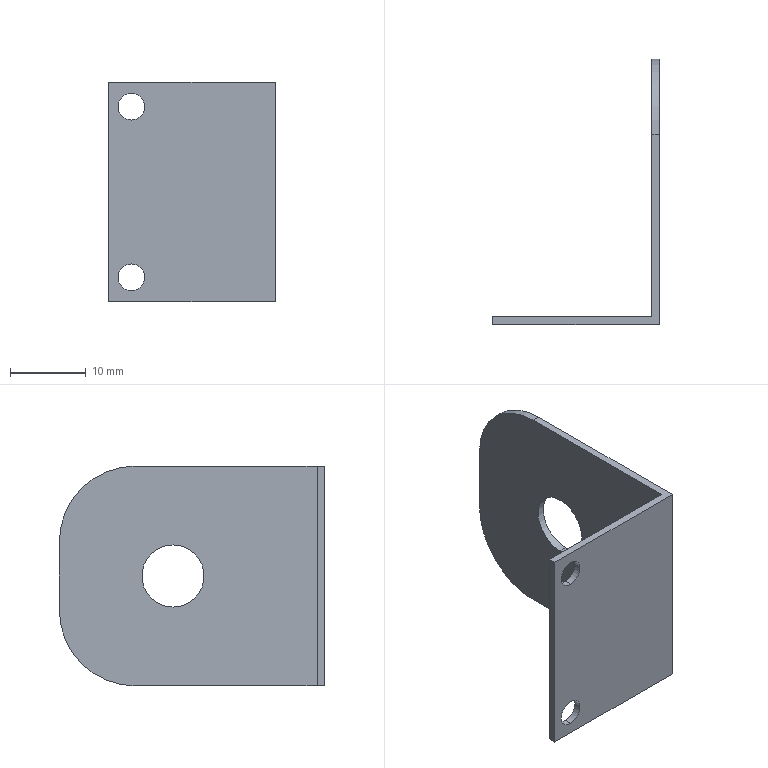Part | 1 solid | 16 faces | box 22 x 35 x 29 mm | volume 1509 mm3 | cylinder 8 | plane 8 | commonest cylinder face diameters 3.5 x4 8.2 x2 20 x2
STEP:
#1=CARTESIAN_POINT('',(10.,20.,4.1));
#2=VERTEX_POINT('',#1);
#3=CARTESIAN_POINT('',(10.,20.,-4.1));
#4=VERTEX_POINT('',#3);
#5=CARTESIAN_POINT('',(10.,20.,0.));
#6=DIRECTION('',(1.,0.,0.));
#7=DIRECTION('',(0.,0.,-1.));
#8=AXIS2_PLACEMENT_3D('',#5,#6,#7);
#9=CIRCLE('',#8,4.1);
#10=EDGE_CURVE('',#2,#4,#9,.T.);
#11=ORIENTED_EDGE('',*,*,#10,.F.);
#12=CARTESIAN_POINT('',(11.,20.,4.1));
#13=VERTEX_POINT('',#12);
#14=CARTESIAN_POINT('',(10.,20.,4.1));
#15=DIRECTION('',(1.,0.,0.));
#16=VECTOR('',#15,1000.);
#17=LINE('',#14,#16);
#18=EDGE_CURVE('',#2,#13,#17,.T.);
#19=ORIENTED_EDGE('',*,*,#18,.T.);
#20=CARTESIAN_POINT('',(11.,20.,-4.1));
#21=VERTEX_POINT('',#20);
#22=CARTESIAN_POINT('',(11.,20.,0.));
#23=DIRECTION('',(1.,0.,0.));
#24=DIRECTION('',(0.,0.,-1.));
#25=AXIS2_PLACEMENT_3D('',#22,#23,#24);
#26=CIRCLE('',#25,4.1);
#27=EDGE_CURVE('',#13,#21,#26,.T.);
#28=ORIENTED_EDGE('',*,*,#27,.T.);
#29=CARTESIAN_POINT('',(10.,20.,-4.1));
#30=DIRECTION('',(1.,0.,0.));
#31=VECTOR('',#30,1000.);
#32=LINE('',#29,#31);
#33=EDGE_CURVE('',#4,#21,#32,.T.);
#34=ORIENTED_EDGE('',*,*,#33,.F.);
#35=EDGE_LOOP('',(#11,#19,#28,#34));
#36=FACE_OUTER_BOUND('',#35,.T.);
#37=CARTESIAN_POINT('',(10.,20.,0.));
#38=DIRECTION('',(1.,0.,0.));
#39=DIRECTION('',(0.,0.,-1.));
#40=AXIS2_PLACEMENT_3D('',#37,#38,#39);
#41=CYLINDRICAL_SURFACE('',#40,4.1);
#42=ADVANCED_FACE('',(#36),#41,.F.);
#43=CARTESIAN_POINT('',(-8.,1.,9.5));
#44=VERTEX_POINT('',#43);
#45=CARTESIAN_POINT('',(-8.,1.,13.));
#46=VERTEX_POINT('',#45);
#47=CARTESIAN_POINT('',(-8.,1.,11.25));
#48=DIRECTION('',(0.,1.,0.));
#49=DIRECTION('',(0.,0.,1.));
#50=AXIS2_PLACEMENT_3D('',#47,#48,#49);
#51=CIRCLE('',#50,1.75);
#52=EDGE_CURVE('',#44,#46,#51,.T.);
#53=ORIENTED_EDGE('',*,*,#52,.T.);
#54=CARTESIAN_POINT('',(-8.,0.,13.));
#55=VERTEX_POINT('',#54);
#56=CARTESIAN_POINT('',(-8.,1.,13.));
#57=DIRECTION('',(0.,-1.,0.));
#58=VECTOR('',#57,1000.);
#59=LINE('',#56,#58);
#60=EDGE_CURVE('',#46,#55,#59,.T.);
#61=ORIENTED_EDGE('',*,*,#60,.T.);
#62=CARTESIAN_POINT('',(-8.,0.,9.5));
#63=VERTEX_POINT('',#62);
#64=CARTESIAN_POINT('',(-8.,0.,11.25));
#65=DIRECTION('',(0.,1.,0.));
#66=DIRECTION('',(0.,0.,1.));
#67=AXIS2_PLACEMENT_3D('',#64,#65,#66);
#68=CIRCLE('',#67,1.75);
#69=EDGE_CURVE('',#63,#55,#68,.T.);
#70=ORIENTED_EDGE('',*,*,#69,.F.);
#71=CARTESIAN_POINT('',(-8.,1.,9.5));
#72=DIRECTION('',(0.,-1.,0.));
#73=VECTOR('',#72,1000.);
#74=LINE('',#71,#73);
#75=EDGE_CURVE('',#44,#63,#74,.T.);
#76=ORIENTED_EDGE('',*,*,#75,.F.);
#77=EDGE_LOOP('',(#53,#61,#70,#76));
#78=FACE_OUTER_BOUND('',#77,.T.);
#79=CARTESIAN_POINT('',(-8.,1.,11.25));
#80=DIRECTION('',(0.,-1.,0.));
#81=DIRECTION('',(0.,0.,-1.));
#82=AXIS2_PLACEMENT_3D('',#79,#80,#81);
#83=CYLINDRICAL_SURFACE('',#82,1.75);
#84=ADVANCED_FACE('',(#78),#83,.F.);
#85=CARTESIAN_POINT('',(-8.,1.,-13.));
#86=VERTEX_POINT('',#85);
#87=CARTESIAN_POINT('',(-8.,1.,-9.5));
#88=VERTEX_POINT('',#87);
#89=CARTESIAN_POINT('',(-8.,1.,-11.25));
#90=DIRECTION('',(0.,1.,0.));
#91=DIRECTION('',(0.,0.,1.));
#92=AXIS2_PLACEMENT_3D('',#89,#90,#91);
#93=CIRCLE('',#92,1.75);
#94=EDGE_CURVE('',#86,#88,#93,.T.);
#95=ORIENTED_EDGE('',*,*,#94,.T.);
#96=CARTESIAN_POINT('',(-8.,0.,-9.5));
#97=VERTEX_POINT('',#96);
#98=CARTESIAN_POINT('',(-8.,1.,-9.5));
#99=DIRECTION('',(0.,-1.,0.));
#100=VECTOR('',#99,1000.);
#101=LINE('',#98,#100);
#102=EDGE_CURVE('',#88,#97,#101,.T.);
#103=ORIENTED_EDGE('',*,*,#102,.T.);
#104=CARTESIAN_POINT('',(-8.,0.,-13.));
#105=VERTEX_POINT('',#104);
#106=CARTESIAN_POINT('',(-8.,0.,-11.25));
#107=DIRECTION('',(0.,1.,0.));
#108=DIRECTION('',(0.,0.,1.));
#109=AXIS2_PLACEMENT_3D('',#106,#107,#108);
#110=CIRCLE('',#109,1.75);
#111=EDGE_CURVE('',#105,#97,#110,.T.);
#112=ORIENTED_EDGE('',*,*,#111,.F.);
#113=CARTESIAN_POINT('',(-8.,1.,-13.));
#114=DIRECTION('',(0.,-1.,0.));
#115=VECTOR('',#114,1000.);
#116=LINE('',#113,#115);
#117=EDGE_CURVE('',#86,#105,#116,.T.);
#118=ORIENTED_EDGE('',*,*,#117,.F.);
#119=EDGE_LOOP('',(#95,#103,#112,#118));
#120=FACE_OUTER_BOUND('',#119,.T.);
#121=CARTESIAN_POINT('',(-8.,1.,-11.25));
#122=DIRECTION('',(0.,-1.,0.));
#123=DIRECTION('',(0.,0.,-1.));
#124=AXIS2_PLACEMENT_3D('',#121,#122,#123);
#125=CYLINDRICAL_SURFACE('',#124,1.75);
#126=ADVANCED_FACE('',(#120),#125,.F.);
#127=CARTESIAN_POINT('',(10.,1.,-14.5));
#128=VERTEX_POINT('',#127);
#129=CARTESIAN_POINT('',(10.,1.,14.5));
#130=VERTEX_POINT('',#129);
#131=CARTESIAN_POINT('',(10.,1.,0.));
#132=DIRECTION('',(0.,0.,1.));
#133=VECTOR('',#132,1000.);
#134=LINE('',#131,#133);
#135=EDGE_CURVE('',#128,#130,#134,.T.);
#136=ORIENTED_EDGE('',*,*,#135,.F.);
#137=CARTESIAN_POINT('',(-11.,1.,-14.5));
#138=VERTEX_POINT('',#137);
#139=CARTESIAN_POINT('',(-11.,1.,-14.5));
#140=DIRECTION('',(-1.,0.,0.));
#141=VECTOR('',#140,1000.);
#142=LINE('',#139,#141);
#143=EDGE_CURVE('',#128,#138,#142,.T.);
#144=ORIENTED_EDGE('',*,*,#143,.T.);
#145=CARTESIAN_POINT('',(-11.,1.,14.5));
#146=VERTEX_POINT('',#145);
#147=CARTESIAN_POINT('',(-11.,1.,-14.5));
#148=DIRECTION('',(0.,0.,1.));
#149=VECTOR('',#148,1000.);
#150=LINE('',#147,#149);
#151=EDGE_CURVE('',#138,#146,#150,.T.);
#152=ORIENTED_EDGE('',*,*,#151,.T.);
#153=CARTESIAN_POINT('',(-11.,1.,14.5));
#154=DIRECTION('',(1.,0.,0.));
#155=VECTOR('',#154,1000.);
#156=LINE('',#153,#155);
#157=EDGE_CURVE('',#146,#130,#156,.T.);
#158=ORIENTED_EDGE('',*,*,#157,.T.);
#159=EDGE_LOOP('',(#136,#144,#152,#158));
#160=FACE_OUTER_BOUND('',#159,.T.);
#161=ORIENTED_EDGE('',*,*,#94,.F.);
#162=CARTESIAN_POINT('',(-8.,1.,-11.25));
#163=DIRECTION('',(0.,1.,0.));
#164=DIRECTION('',(0.,0.,1.));
#165=AXIS2_PLACEMENT_3D('',#162,#163,#164);
#166=CIRCLE('',#165,1.75);
#167=EDGE_CURVE('',#88,#86,#166,.T.);
#168=ORIENTED_EDGE('',*,*,#167,.F.);
#169=EDGE_LOOP('',(#161,#168));
#170=FACE_BOUND('',#169,.T.);
#171=ORIENTED_EDGE('',*,*,#52,.F.);
#172=CARTESIAN_POINT('',(-8.,1.,11.25));
#173=DIRECTION('',(0.,1.,0.));
#174=DIRECTION('',(0.,0.,1.));
#175=AXIS2_PLACEMENT_3D('',#172,#173,#174);
#176=CIRCLE('',#175,1.75);
#177=EDGE_CURVE('',#46,#44,#176,.T.);
#178=ORIENTED_EDGE('',*,*,#177,.F.);
#179=EDGE_LOOP('',(#171,#178));
#180=FACE_BOUND('',#179,.T.);
#181=CARTESIAN_POINT('',(0.,1.,0.));
#182=DIRECTION('',(0.,1.,0.));
#183=DIRECTION('',(0.,0.,1.));
#184=AXIS2_PLACEMENT_3D('',#181,#182,#183);
#185=PLANE('',#184);
#186=ADVANCED_FACE('',(#160,#170,#180),#185,.T.);
#187=CARTESIAN_POINT('',(-11.,0.,-14.5));
#188=VERTEX_POINT('',#187);
#189=CARTESIAN_POINT('',(-11.,0.,14.5));
#190=VERTEX_POINT('',#189);
#191=CARTESIAN_POINT('',(-11.,0.,-14.5));
#192=DIRECTION('',(0.,0.,1.));
#193=VECTOR('',#192,1000.);
#194=LINE('',#191,#193);
#195=EDGE_CURVE('',#188,#190,#194,.T.);
#196=ORIENTED_EDGE('',*,*,#195,.F.);
#197=CARTESIAN_POINT('',(11.,0.,-14.5));
#198=VERTEX_POINT('',#197);
#199=CARTESIAN_POINT('',(-11.,0.,-14.5));
#200=DIRECTION('',(-1.,0.,0.));
#201=VECTOR('',#200,1000.);
#202=LINE('',#199,#201);
#203=EDGE_CURVE('',#198,#188,#202,.T.);
#204=ORIENTED_EDGE('',*,*,#203,.F.);
#205=CARTESIAN_POINT('',(11.,0.,14.5));
#206=VERTEX_POINT('',#205);
#207=CARTESIAN_POINT('',(11.,0.,-14.5));
#208=DIRECTION('',(0.,0.,-1.));
#209=VECTOR('',#208,1000.);
#210=LINE('',#207,#209);
#211=EDGE_CURVE('',#206,#198,#210,.T.);
#212=ORIENTED_EDGE('',*,*,#211,.F.);
#213=CARTESIAN_POINT('',(-11.,0.,14.5));
#214=DIRECTION('',(1.,0.,0.));
#215=VECTOR('',#214,1000.);
#216=LINE('',#213,#215);
#217=EDGE_CURVE('',#190,#206,#216,.T.);
#218=ORIENTED_EDGE('',*,*,#217,.F.);
#219=EDGE_LOOP('',(#196,#204,#212,#218));
#220=FACE_OUTER_BOUND('',#219,.T.);
#221=ORIENTED_EDGE('',*,*,#111,.T.);
#222=CARTESIAN_POINT('',(-8.,0.,-11.25));
#223=DIRECTION('',(0.,1.,0.));
#224=DIRECTION('',(0.,0.,1.));
#225=AXIS2_PLACEMENT_3D('',#222,#223,#224);
#226=CIRCLE('',#225,1.75);
#227=EDGE_CURVE('',#97,#105,#226,.T.);
#228=ORIENTED_EDGE('',*,*,#227,.T.);
#229=EDGE_LOOP('',(#221,#228));
#230=FACE_BOUND('',#229,.T.);
#231=ORIENTED_EDGE('',*,*,#69,.T.);
#232=CARTESIAN_POINT('',(-8.,0.,11.25));
#233=DIRECTION('',(0.,1.,0.));
#234=DIRECTION('',(0.,0.,1.));
#235=AXIS2_PLACEMENT_3D('',#232,#233,#234);
#236=CIRCLE('',#235,1.75);
#237=EDGE_CURVE('',#55,#63,#236,.T.);
#238=ORIENTED_EDGE('',*,*,#237,.T.);
#239=EDGE_LOOP('',(#231,#238));
#240=FACE_BOUND('',#239,.T.);
#241=CARTESIAN_POINT('',(0.,0.,0.));
#242=DIRECTION('',(0.,1.,0.));
#243=DIRECTION('',(0.,0.,1.));
#244=AXIS2_PLACEMENT_3D('',#241,#242,#243);
#245=PLANE('',#244);
#246=ADVANCED_FACE('',(#220,#230,#240),#245,.F.);
#247=CARTESIAN_POINT('',(11.,25.,-14.5));
#248=VERTEX_POINT('',#247);
#249=CARTESIAN_POINT('',(11.,1.,-14.5));
#250=DIRECTION('',(0.,-1.,0.));
#251=VECTOR('',#250,1000.);
#252=LINE('',#249,#251);
#253=EDGE_CURVE('',#248,#198,#252,.T.);
#254=ORIENTED_EDGE('',*,*,#253,.F.);
#255=CARTESIAN_POINT('',(11.,35.,-4.5));
#256=VERTEX_POINT('',#255);
#257=CARTESIAN_POINT('',(11.,25.,-4.5));
#258=DIRECTION('',(1.,0.,0.));
#259=DIRECTION('',(0.,0.,1.));
#260=AXIS2_PLACEMENT_3D('',#257,#258,#259);
#261=CIRCLE('',#260,10.);
#262=EDGE_CURVE('',#248,#256,#261,.T.);
#263=ORIENTED_EDGE('',*,*,#262,.T.);
#264=CARTESIAN_POINT('',(11.,35.,4.5));
#265=VERTEX_POINT('',#264);
#266=CARTESIAN_POINT('',(11.,35.,14.5));
#267=DIRECTION('',(0.,0.,1.));
#268=VECTOR('',#267,1000.);
#269=LINE('',#266,#268);
#270=EDGE_CURVE('',#256,#265,#269,.T.);
#271=ORIENTED_EDGE('',*,*,#270,.T.);
#272=CARTESIAN_POINT('',(11.,25.,14.5));
#273=VERTEX_POINT('',#272);
#274=CARTESIAN_POINT('',(11.,25.,4.5));
#275=DIRECTION('',(1.,0.,0.));
#276=DIRECTION('',(0.,0.,1.));
#277=AXIS2_PLACEMENT_3D('',#274,#275,#276);
#278=CIRCLE('',#277,10.);
#279=EDGE_CURVE('',#265,#273,#278,.T.);
#280=ORIENTED_EDGE('',*,*,#279,.T.);
#281=CARTESIAN_POINT('',(11.,1.,14.5));
#282=DIRECTION('',(0.,-1.,0.));
#283=VECTOR('',#282,1000.);
#284=LINE('',#281,#283);
#285=EDGE_CURVE('',#273,#206,#284,.T.);
#286=ORIENTED_EDGE('',*,*,#285,.T.);
#287=ORIENTED_EDGE('',*,*,#211,.T.);
#288=EDGE_LOOP('',(#254,#263,#271,#280,#286,#287));
#289=FACE_OUTER_BOUND('',#288,.T.);
#290=CARTESIAN_POINT('',(11.,20.,0.));
#291=DIRECTION('',(1.,0.,0.));
#292=DIRECTION('',(0.,0.,-1.));
#293=AXIS2_PLACEMENT_3D('',#290,#291,#292);
#294=CIRCLE('',#293,4.1);
#295=EDGE_CURVE('',#21,#13,#294,.T.);
#296=ORIENTED_EDGE('',*,*,#295,.F.);
#297=ORIENTED_EDGE('',*,*,#27,.F.);
#298=EDGE_LOOP('',(#296,#297));
#299=FACE_BOUND('',#298,.T.);
#300=CARTESIAN_POINT('',(11.,1.,-14.5));
#301=DIRECTION('',(-1.,0.,0.));
#302=DIRECTION('',(0.,0.,1.));
#303=AXIS2_PLACEMENT_3D('',#300,#301,#302);
#304=PLANE('',#303);
#305=ADVANCED_FACE('',(#289,#299),#304,.F.);
#306=CARTESIAN_POINT('',(10.,25.,-14.5));
#307=VERTEX_POINT('',#306);
#308=CARTESIAN_POINT('',(10.,0.,-14.5));
#309=DIRECTION('',(0.,1.,0.));
#310=VECTOR('',#309,1000.);
#311=LINE('',#308,#310);
#312=EDGE_CURVE('',#128,#307,#311,.T.);
#313=ORIENTED_EDGE('',*,*,#312,.T.);
#314=CARTESIAN_POINT('',(11.,25.,-14.5));
#315=DIRECTION('',(1.,0.,0.));
#316=VECTOR('',#315,1000.);
#317=LINE('',#314,#316);
#318=EDGE_CURVE('',#307,#248,#317,.T.);
#319=ORIENTED_EDGE('',*,*,#318,.T.);
#320=ORIENTED_EDGE('',*,*,#253,.T.);
#321=ORIENTED_EDGE('',*,*,#203,.T.);
#322=CARTESIAN_POINT('',(-11.,1.,-14.5));
#323=DIRECTION('',(0.,-1.,0.));
#324=VECTOR('',#323,1000.);
#325=LINE('',#322,#324);
#326=EDGE_CURVE('',#138,#188,#325,.T.);
#327=ORIENTED_EDGE('',*,*,#326,.F.);
#328=ORIENTED_EDGE('',*,*,#143,.F.);
#329=EDGE_LOOP('',(#313,#319,#320,#321,#327,#328));
#330=FACE_OUTER_BOUND('',#329,.T.);
#331=CARTESIAN_POINT('',(-11.,1.,-14.5));
#332=DIRECTION('',(0.,0.,1.));
#333=DIRECTION('',(1.,0.,0.));
#334=AXIS2_PLACEMENT_3D('',#331,#332,#333);
#335=PLANE('',#334);
#336=ADVANCED_FACE('',(#330),#335,.F.);
#337=ORIENTED_EDGE('',*,*,#195,.T.);
#338=CARTESIAN_POINT('',(-11.,1.,14.5));
#339=DIRECTION('',(0.,-1.,0.));
#340=VECTOR('',#339,1000.);
#341=LINE('',#338,#340);
#342=EDGE_CURVE('',#146,#190,#341,.T.);
#343=ORIENTED_EDGE('',*,*,#342,.F.);
#344=ORIENTED_EDGE('',*,*,#151,.F.);
#345=ORIENTED_EDGE('',*,*,#326,.T.);
#346=EDGE_LOOP('',(#337,#343,#344,#345));
#347=FACE_OUTER_BOUND('',#346,.T.);
#348=CARTESIAN_POINT('',(-11.,1.,-14.5));
#349=DIRECTION('',(1.,0.,0.));
#350=DIRECTION('',(0.,0.,-1.));
#351=AXIS2_PLACEMENT_3D('',#348,#349,#350);
#352=PLANE('',#351);
#353=ADVANCED_FACE('',(#347),#352,.F.);
#354=ORIENTED_EDGE('',*,*,#285,.F.);
#355=CARTESIAN_POINT('',(10.,25.,14.5));
#356=VERTEX_POINT('',#355);
#357=CARTESIAN_POINT('',(10.,25.,14.5));
#358=DIRECTION('',(-1.,0.,0.));
#359=VECTOR('',#358,1000.);
#360=LINE('',#357,#359);
#361=EDGE_CURVE('',#273,#356,#360,.T.);
#362=ORIENTED_EDGE('',*,*,#361,.T.);
#363=CARTESIAN_POINT('',(10.,0.,14.5));
#364=DIRECTION('',(0.,-1.,0.));
#365=VECTOR('',#364,1000.);
#366=LINE('',#363,#365);
#367=EDGE_CURVE('',#356,#130,#366,.T.);
#368=ORIENTED_EDGE('',*,*,#367,.T.);
#369=ORIENTED_EDGE('',*,*,#157,.F.);
#370=ORIENTED_EDGE('',*,*,#342,.T.);
#371=ORIENTED_EDGE('',*,*,#217,.T.);
#372=EDGE_LOOP('',(#354,#362,#368,#369,#370,#371));
#373=FACE_OUTER_BOUND('',#372,.T.);
#374=CARTESIAN_POINT('',(-11.,1.,14.5));
#375=DIRECTION('',(0.,0.,-1.));
#376=DIRECTION('',(-1.,0.,0.));
#377=AXIS2_PLACEMENT_3D('',#374,#375,#376);
#378=PLANE('',#377);
#379=ADVANCED_FACE('',(#373),#378,.F.);
#380=ORIENTED_EDGE('',*,*,#102,.F.);
#381=ORIENTED_EDGE('',*,*,#167,.T.);
#382=ORIENTED_EDGE('',*,*,#117,.T.);
#383=ORIENTED_EDGE('',*,*,#227,.F.);
#384=EDGE_LOOP('',(#380,#381,#382,#383));
#385=FACE_OUTER_BOUND('',#384,.T.);
#386=CARTESIAN_POINT('',(-8.,1.,-11.25));
#387=DIRECTION('',(0.,-1.,0.));
#388=DIRECTION('',(0.,0.,-1.));
#389=AXIS2_PLACEMENT_3D('',#386,#387,#388);
#390=CYLINDRICAL_SURFACE('',#389,1.75);
#391=ADVANCED_FACE('',(#385),#390,.F.);
#392=ORIENTED_EDGE('',*,*,#60,.F.);
#393=ORIENTED_EDGE('',*,*,#177,.T.);
#394=ORIENTED_EDGE('',*,*,#75,.T.);
#395=ORIENTED_EDGE('',*,*,#237,.F.);
#396=EDGE_LOOP('',(#392,#393,#394,#395));
#397=FACE_OUTER_BOUND('',#396,.T.);
#398=CARTESIAN_POINT('',(-8.,1.,11.25));
#399=DIRECTION('',(0.,-1.,0.));
#400=DIRECTION('',(0.,0.,-1.));
#401=AXIS2_PLACEMENT_3D('',#398,#399,#400);
#402=CYLINDRICAL_SURFACE('',#401,1.75);
#403=ADVANCED_FACE('',(#397),#402,.F.);
#404=ORIENTED_EDGE('',*,*,#270,.F.);
#405=CARTESIAN_POINT('',(10.,35.,-4.5));
#406=VERTEX_POINT('',#405);
#407=CARTESIAN_POINT('',(10.,35.,-4.5));
#408=DIRECTION('',(-1.,0.,0.));
#409=VECTOR('',#408,1000.);
#410=LINE('',#407,#409);
#411=EDGE_CURVE('',#256,#406,#410,.T.);
#412=ORIENTED_EDGE('',*,*,#411,.T.);
#413=CARTESIAN_POINT('',(10.,35.,4.5));
#414=VERTEX_POINT('',#413);
#415=CARTESIAN_POINT('',(10.,35.,14.5));
#416=DIRECTION('',(0.,0.,1.));
#417=VECTOR('',#416,1000.);
#418=LINE('',#415,#417);
#419=EDGE_CURVE('',#406,#414,#418,.T.);
#420=ORIENTED_EDGE('',*,*,#419,.T.);
#421=CARTESIAN_POINT('',(11.,35.,4.5));
#422=DIRECTION('',(1.,0.,0.));
#423=VECTOR('',#422,1000.);
#424=LINE('',#421,#423);
#425=EDGE_CURVE('',#414,#265,#424,.T.);
#426=ORIENTED_EDGE('',*,*,#425,.T.);
#427=EDGE_LOOP('',(#404,#412,#420,#426));
#428=FACE_OUTER_BOUND('',#427,.T.);
#429=CARTESIAN_POINT('',(10.,35.,14.5));
#430=DIRECTION('',(0.,1.,0.));
#431=DIRECTION('',(0.,0.,1.));
#432=AXIS2_PLACEMENT_3D('',#429,#430,#431);
#433=PLANE('',#432);
#434=ADVANCED_FACE('',(#428),#433,.T.);
#435=CARTESIAN_POINT('',(10.,20.,0.));
#436=DIRECTION('',(1.,0.,0.));
#437=DIRECTION('',(0.,0.,-1.));
#438=AXIS2_PLACEMENT_3D('',#435,#436,#437);
#439=CIRCLE('',#438,4.1);
#440=EDGE_CURVE('',#4,#2,#439,.T.);
#441=ORIENTED_EDGE('',*,*,#440,.T.);
#442=ORIENTED_EDGE('',*,*,#10,.T.);
#443=EDGE_LOOP('',(#441,#442));
#444=FACE_BOUND('',#443,.T.);
#445=ORIENTED_EDGE('',*,*,#419,.F.);
#446=CARTESIAN_POINT('',(10.,25.,-4.5));
#447=DIRECTION('',(-1.,0.,0.));
#448=DIRECTION('',(0.,0.,1.));
#449=AXIS2_PLACEMENT_3D('',#446,#447,#448);
#450=CIRCLE('',#449,10.);
#451=EDGE_CURVE('',#406,#307,#450,.T.);
#452=ORIENTED_EDGE('',*,*,#451,.T.);
#453=ORIENTED_EDGE('',*,*,#312,.F.);
#454=ORIENTED_EDGE('',*,*,#135,.T.);
#455=ORIENTED_EDGE('',*,*,#367,.F.);
#456=CARTESIAN_POINT('',(10.,25.,4.5));
#457=DIRECTION('',(-1.,0.,0.));
#458=DIRECTION('',(0.,0.,1.));
#459=AXIS2_PLACEMENT_3D('',#456,#457,#458);
#460=CIRCLE('',#459,10.);
#461=EDGE_CURVE('',#356,#414,#460,.T.);
#462=ORIENTED_EDGE('',*,*,#461,.T.);
#463=EDGE_LOOP('',(#445,#452,#453,#454,#455,#462));
#464=FACE_OUTER_BOUND('',#463,.T.);
#465=CARTESIAN_POINT('',(10.,0.,0.));
#466=DIRECTION('',(-1.,0.,0.));
#467=DIRECTION('',(0.,0.,1.));
#468=AXIS2_PLACEMENT_3D('',#465,#466,#467);
#469=PLANE('',#468);
#470=ADVANCED_FACE('',(#444,#464),#469,.T.);
#471=ORIENTED_EDGE('',*,*,#18,.F.);
#472=ORIENTED_EDGE('',*,*,#440,.F.);
#473=ORIENTED_EDGE('',*,*,#33,.T.);
#474=ORIENTED_EDGE('',*,*,#295,.T.);
#475=EDGE_LOOP('',(#471,#472,#473,#474));
#476=FACE_OUTER_BOUND('',#475,.T.);
#477=CARTESIAN_POINT('',(10.,20.,0.));
#478=DIRECTION('',(1.,0.,0.));
#479=DIRECTION('',(0.,0.,-1.));
#480=AXIS2_PLACEMENT_3D('',#477,#478,#479);
#481=CYLINDRICAL_SURFACE('',#480,4.1);
#482=ADVANCED_FACE('',(#476),#481,.F.);
#483=ORIENTED_EDGE('',*,*,#451,.F.);
#484=ORIENTED_EDGE('',*,*,#411,.F.);
#485=ORIENTED_EDGE('',*,*,#262,.F.);
#486=ORIENTED_EDGE('',*,*,#318,.F.);
#487=EDGE_LOOP('',(#483,#484,#485,#486));
#488=FACE_OUTER_BOUND('',#487,.T.);
#489=CARTESIAN_POINT('',(-11.,25.,-4.5));
#490=DIRECTION('',(-1.,0.,0.));
#491=DIRECTION('',(0.,0.,1.));
#492=AXIS2_PLACEMENT_3D('',#489,#490,#491);
#493=CYLINDRICAL_SURFACE('',#492,10.);
#494=ADVANCED_FACE('',(#488),#493,.T.);
#495=ORIENTED_EDGE('',*,*,#461,.F.);
#496=ORIENTED_EDGE('',*,*,#361,.F.);
#497=ORIENTED_EDGE('',*,*,#279,.F.);
#498=ORIENTED_EDGE('',*,*,#425,.F.);
#499=EDGE_LOOP('',(#495,#496,#497,#498));
#500=FACE_OUTER_BOUND('',#499,.T.);
#501=CARTESIAN_POINT('',(10.,25.,4.5));
#502=DIRECTION('',(-1.,0.,0.));
#503=DIRECTION('',(0.,0.,1.));
#504=AXIS2_PLACEMENT_3D('',#501,#502,#503);
#505=CYLINDRICAL_SURFACE('',#504,10.);
#506=ADVANCED_FACE('',(#500),#505,.T.);
#507=CLOSED_SHELL('',(#42,#84,#126,#186,#246,#305,#336,#353,#379,#391,#403,#434,#470,#482,#494,#506));
#508=MANIFOLD_SOLID_BREP('',#507);
#509=CARTESIAN_POINT('',(0.,0.,0.));
#510=DIRECTION('',(0.,0.,1.));
#511=DIRECTION('',(1.,0.,0.));
#512=AXIS2_PLACEMENT_3D('',#509,#510,#511);
#513=(LENGTH_UNIT()NAMED_UNIT(*)SI_UNIT(.MILLI.,.METRE.));
#514=UNCERTAINTY_MEASURE_WITH_UNIT(LENGTH_MEASURE(0.00001),#513,'','');
#515=(NAMED_UNIT(*)PLANE_ANGLE_UNIT()SI_UNIT($,.RADIAN.));
#516=(NAMED_UNIT(*)SI_UNIT($,.STERADIAN.)SOLID_ANGLE_UNIT());
#517=(GEOMETRIC_REPRESENTATION_CONTEXT(3)GLOBAL_UNCERTAINTY_ASSIGNED_CONTEXT((#514))GLOBAL_UNIT_ASSIGNED_CONTEXT((#513,#515,#516))REPRESENTATION_CONTEXT('',''));
#518=ADVANCED_BREP_SHAPE_REPRESENTATION('',(#508,#512),#517);